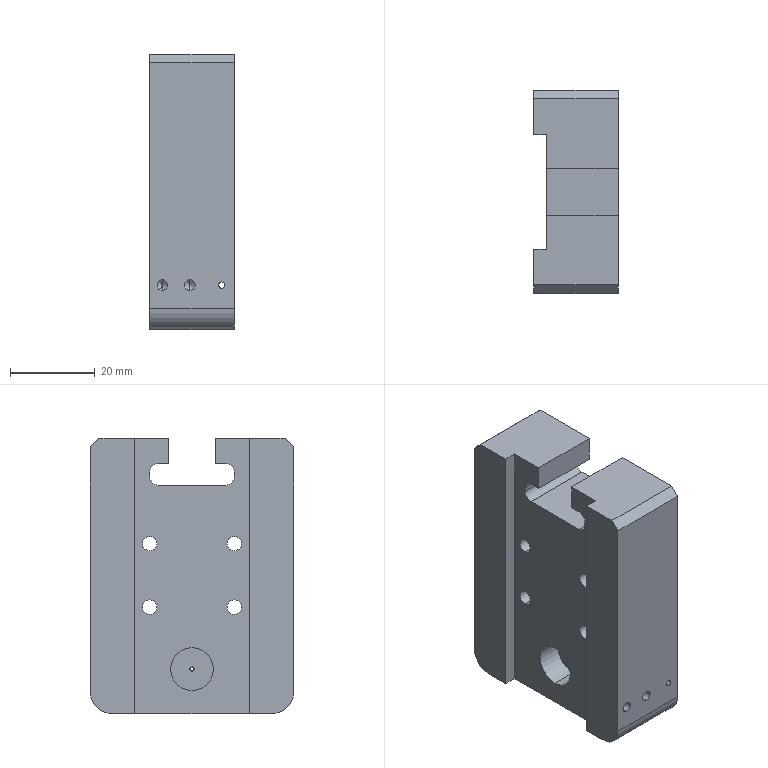Part | SolidWorks | features ICE 6, HoleWzd 3, Chamfer 2, Fillet 2, Extrusion 1, MoveFace 1 | 1 solid | 84 faces | box 20 x 48 x 65 mm | volume 52206 mm3 | cylinder 44 | plane 26 | cone 14 | commonest cylinder face diameters 2.5 x12 3.4 x8 6 x8 1.5 x4 4 x4 1 x2